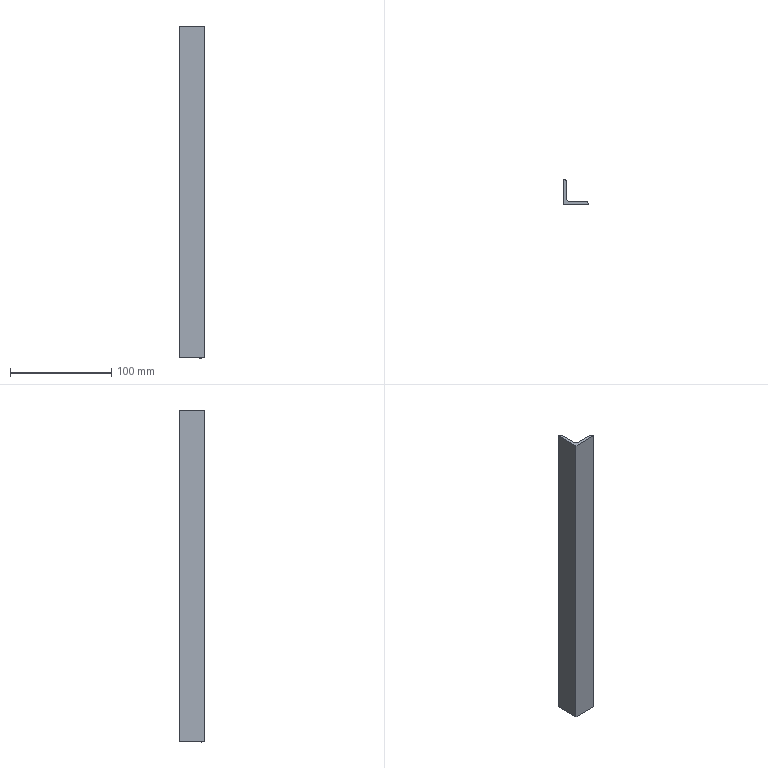Part | SolidWorks | features BaseBody 1 | 1 solid | 9 faces | box 25 x 25 x 328 mm | volume 45614 mm3 | plane 6 | cylinder 3 | commonest cylinder face diameters 6 x3
STEP:
#1=CARTESIAN_POINT('',(3.,22.,164.));
#2=VERTEX_POINT('',#1);
#3=CARTESIAN_POINT('',(0.,25.,164.));
#4=VERTEX_POINT('',#3);
#5=CARTESIAN_POINT('',(0.,22.,164.));
#6=DIRECTION('',(0.,0.,1.));
#7=DIRECTION('',(-1.,0.,0.));
#8=AXIS2_PLACEMENT_3D('',#5,#6,#7);
#9=CIRCLE('',#8,3.);
#10=EDGE_CURVE('',#2,#4,#9,.T.);
#11=ORIENTED_EDGE('',*,*,#10,.F.);
#12=CARTESIAN_POINT('',(3.,22.,-164.));
#13=VERTEX_POINT('',#12);
#14=CARTESIAN_POINT('',(3.,22.,164.));
#15=DIRECTION('',(0.,0.,1.));
#16=VECTOR('',#15,1000.);
#17=LINE('',#14,#16);
#18=EDGE_CURVE('',#13,#2,#17,.T.);
#19=ORIENTED_EDGE('',*,*,#18,.F.);
#20=CARTESIAN_POINT('',(0.,25.,-164.));
#21=VERTEX_POINT('',#20);
#22=CARTESIAN_POINT('',(0.,22.,-164.));
#23=DIRECTION('',(0.,0.,-1.));
#24=DIRECTION('',(-1.,0.,0.));
#25=AXIS2_PLACEMENT_3D('',#22,#23,#24);
#26=CIRCLE('',#25,3.);
#27=EDGE_CURVE('',#21,#13,#26,.T.);
#28=ORIENTED_EDGE('',*,*,#27,.F.);
#29=CARTESIAN_POINT('',(0.,25.,164.));
#30=DIRECTION('',(0.,0.,-1.));
#31=VECTOR('',#30,1000.);
#32=LINE('',#29,#31);
#33=EDGE_CURVE('',#4,#21,#32,.T.);
#34=ORIENTED_EDGE('',*,*,#33,.F.);
#35=EDGE_LOOP('',(#11,#19,#28,#34));
#36=FACE_OUTER_BOUND('',#35,.T.);
#37=CARTESIAN_POINT('',(0.,22.,164.));
#38=DIRECTION('',(0.,0.,-1.));
#39=DIRECTION('',(-1.,0.,0.));
#40=AXIS2_PLACEMENT_3D('',#37,#38,#39);
#41=CYLINDRICAL_SURFACE('',#40,3.);
#42=ADVANCED_FACE('',(#36),#41,.T.);
#43=CARTESIAN_POINT('',(25.,0.,164.));
#44=VERTEX_POINT('',#43);
#45=CARTESIAN_POINT('',(22.,3.,164.));
#46=VERTEX_POINT('',#45);
#47=CARTESIAN_POINT('',(22.,0.,164.));
#48=DIRECTION('',(0.,0.,1.));
#49=DIRECTION('',(-1.,0.,0.));
#50=AXIS2_PLACEMENT_3D('',#47,#48,#49);
#51=CIRCLE('',#50,3.);
#52=EDGE_CURVE('',#44,#46,#51,.T.);
#53=ORIENTED_EDGE('',*,*,#52,.F.);
#54=CARTESIAN_POINT('',(25.,0.,-164.));
#55=VERTEX_POINT('',#54);
#56=CARTESIAN_POINT('',(25.,0.,164.));
#57=DIRECTION('',(0.,0.,-1.));
#58=VECTOR('',#57,1000.);
#59=LINE('',#56,#58);
#60=EDGE_CURVE('',#44,#55,#59,.T.);
#61=ORIENTED_EDGE('',*,*,#60,.T.);
#62=CARTESIAN_POINT('',(22.,3.,-164.));
#63=VERTEX_POINT('',#62);
#64=CARTESIAN_POINT('',(22.,0.,-164.));
#65=DIRECTION('',(0.,0.,-1.));
#66=DIRECTION('',(-1.,0.,0.));
#67=AXIS2_PLACEMENT_3D('',#64,#65,#66);
#68=CIRCLE('',#67,3.);
#69=EDGE_CURVE('',#63,#55,#68,.T.);
#70=ORIENTED_EDGE('',*,*,#69,.F.);
#71=CARTESIAN_POINT('',(22.,3.,164.));
#72=DIRECTION('',(0.,0.,-1.));
#73=VECTOR('',#72,1000.);
#74=LINE('',#71,#73);
#75=EDGE_CURVE('',#46,#63,#74,.T.);
#76=ORIENTED_EDGE('',*,*,#75,.F.);
#77=EDGE_LOOP('',(#53,#61,#70,#76));
#78=FACE_OUTER_BOUND('',#77,.T.);
#79=CARTESIAN_POINT('',(22.,0.,164.));
#80=DIRECTION('',(0.,0.,-1.));
#81=DIRECTION('',(-1.,0.,0.));
#82=AXIS2_PLACEMENT_3D('',#79,#80,#81);
#83=CYLINDRICAL_SURFACE('',#82,3.);
#84=ADVANCED_FACE('',(#78),#83,.T.);
#85=CARTESIAN_POINT('',(6.,3.,164.));
#86=VERTEX_POINT('',#85);
#87=CARTESIAN_POINT('',(3.,6.,164.));
#88=VERTEX_POINT('',#87);
#89=CARTESIAN_POINT('',(6.,6.,164.));
#90=DIRECTION('',(0.,0.,-1.));
#91=DIRECTION('',(-1.,0.,0.));
#92=AXIS2_PLACEMENT_3D('',#89,#90,#91);
#93=CIRCLE('',#92,3.);
#94=EDGE_CURVE('',#86,#88,#93,.T.);
#95=ORIENTED_EDGE('',*,*,#94,.F.);
#96=CARTESIAN_POINT('',(6.,3.,-164.));
#97=VERTEX_POINT('',#96);
#98=CARTESIAN_POINT('',(6.,3.,164.));
#99=DIRECTION('',(0.,0.,1.));
#100=VECTOR('',#99,1000.);
#101=LINE('',#98,#100);
#102=EDGE_CURVE('',#97,#86,#101,.T.);
#103=ORIENTED_EDGE('',*,*,#102,.F.);
#104=CARTESIAN_POINT('',(3.,6.,-164.));
#105=VERTEX_POINT('',#104);
#106=CARTESIAN_POINT('',(6.,6.,-164.));
#107=DIRECTION('',(0.,0.,1.));
#108=DIRECTION('',(-1.,0.,0.));
#109=AXIS2_PLACEMENT_3D('',#106,#107,#108);
#110=CIRCLE('',#109,3.);
#111=EDGE_CURVE('',#105,#97,#110,.T.);
#112=ORIENTED_EDGE('',*,*,#111,.F.);
#113=CARTESIAN_POINT('',(3.,6.,-164.));
#114=DIRECTION('',(0.,0.,-1.));
#115=VECTOR('',#114,1000.);
#116=LINE('',#113,#115);
#117=EDGE_CURVE('',#88,#105,#116,.T.);
#118=ORIENTED_EDGE('',*,*,#117,.F.);
#119=EDGE_LOOP('',(#95,#103,#112,#118));
#120=FACE_OUTER_BOUND('',#119,.T.);
#121=CARTESIAN_POINT('',(6.,6.,164.));
#122=DIRECTION('',(0.,0.,1.));
#123=DIRECTION('',(1.,0.,0.));
#124=AXIS2_PLACEMENT_3D('',#121,#122,#123);
#125=CYLINDRICAL_SURFACE('',#124,3.);
#126=ADVANCED_FACE('',(#120),#125,.F.);
#127=CARTESIAN_POINT('',(3.,3.,-164.));
#128=DIRECTION('',(-1.,0.,0.));
#129=VECTOR('',#128,1000.);
#130=LINE('',#127,#129);
#131=EDGE_CURVE('',#63,#97,#130,.T.);
#132=ORIENTED_EDGE('',*,*,#131,.F.);
#133=ORIENTED_EDGE('',*,*,#69,.T.);
#134=CARTESIAN_POINT('',(0.,0.,-164.));
#135=VERTEX_POINT('',#134);
#136=CARTESIAN_POINT('',(0.,0.,-164.));
#137=DIRECTION('',(1.,0.,0.));
#138=VECTOR('',#137,1000.);
#139=LINE('',#136,#138);
#140=EDGE_CURVE('',#135,#55,#139,.T.);
#141=ORIENTED_EDGE('',*,*,#140,.F.);
#142=CARTESIAN_POINT('',(0.,0.,-164.));
#143=DIRECTION('',(0.,-1.,0.));
#144=VECTOR('',#143,1000.);
#145=LINE('',#142,#144);
#146=EDGE_CURVE('',#21,#135,#145,.T.);
#147=ORIENTED_EDGE('',*,*,#146,.F.);
#148=ORIENTED_EDGE('',*,*,#27,.T.);
#149=CARTESIAN_POINT('',(3.,25.,-164.));
#150=DIRECTION('',(0.,1.,0.));
#151=VECTOR('',#150,1000.);
#152=LINE('',#149,#151);
#153=EDGE_CURVE('',#105,#13,#152,.T.);
#154=ORIENTED_EDGE('',*,*,#153,.F.);
#155=ORIENTED_EDGE('',*,*,#111,.T.);
#156=EDGE_LOOP('',(#132,#133,#141,#147,#148,#154,#155));
#157=FACE_OUTER_BOUND('',#156,.T.);
#158=CARTESIAN_POINT('',(0.,0.,-164.));
#159=DIRECTION('',(0.,0.,-1.));
#160=DIRECTION('',(0.,-1.,0.));
#161=AXIS2_PLACEMENT_3D('',#158,#159,#160);
#162=PLANE('',#161);
#163=ADVANCED_FACE('',(#157),#162,.T.);
#164=CARTESIAN_POINT('',(0.,0.,164.));
#165=VERTEX_POINT('',#164);
#166=CARTESIAN_POINT('',(0.,0.,164.));
#167=DIRECTION('',(1.,0.,0.));
#168=VECTOR('',#167,1000.);
#169=LINE('',#166,#168);
#170=EDGE_CURVE('',#165,#44,#169,.T.);
#171=ORIENTED_EDGE('',*,*,#170,.T.);
#172=ORIENTED_EDGE('',*,*,#52,.T.);
#173=CARTESIAN_POINT('',(3.,3.,164.));
#174=DIRECTION('',(-1.,0.,0.));
#175=VECTOR('',#174,1000.);
#176=LINE('',#173,#175);
#177=EDGE_CURVE('',#46,#86,#176,.T.);
#178=ORIENTED_EDGE('',*,*,#177,.T.);
#179=ORIENTED_EDGE('',*,*,#94,.T.);
#180=CARTESIAN_POINT('',(3.,25.,164.));
#181=DIRECTION('',(0.,1.,0.));
#182=VECTOR('',#181,1000.);
#183=LINE('',#180,#182);
#184=EDGE_CURVE('',#88,#2,#183,.T.);
#185=ORIENTED_EDGE('',*,*,#184,.T.);
#186=ORIENTED_EDGE('',*,*,#10,.T.);
#187=CARTESIAN_POINT('',(0.,0.,164.));
#188=DIRECTION('',(0.,-1.,0.));
#189=VECTOR('',#188,1000.);
#190=LINE('',#187,#189);
#191=EDGE_CURVE('',#4,#165,#190,.T.);
#192=ORIENTED_EDGE('',*,*,#191,.T.);
#193=EDGE_LOOP('',(#171,#172,#178,#179,#185,#186,#192));
#194=FACE_OUTER_BOUND('',#193,.T.);
#195=CARTESIAN_POINT('',(0.,0.,164.));
#196=DIRECTION('',(0.,0.,-1.));
#197=DIRECTION('',(0.,-1.,0.));
#198=AXIS2_PLACEMENT_3D('',#195,#196,#197);
#199=PLANE('',#198);
#200=ADVANCED_FACE('',(#194),#199,.F.);
#201=ORIENTED_EDGE('',*,*,#153,.T.);
#202=ORIENTED_EDGE('',*,*,#18,.T.);
#203=ORIENTED_EDGE('',*,*,#184,.F.);
#204=ORIENTED_EDGE('',*,*,#117,.T.);
#205=EDGE_LOOP('',(#201,#202,#203,#204));
#206=FACE_OUTER_BOUND('',#205,.T.);
#207=CARTESIAN_POINT('',(3.,25.,164.));
#208=DIRECTION('',(-1.,0.,0.));
#209=DIRECTION('',(0.,1.,0.));
#210=AXIS2_PLACEMENT_3D('',#207,#208,#209);
#211=PLANE('',#210);
#212=ADVANCED_FACE('',(#206),#211,.F.);
#213=ORIENTED_EDGE('',*,*,#177,.F.);
#214=ORIENTED_EDGE('',*,*,#75,.T.);
#215=ORIENTED_EDGE('',*,*,#131,.T.);
#216=ORIENTED_EDGE('',*,*,#102,.T.);
#217=EDGE_LOOP('',(#213,#214,#215,#216));
#218=FACE_OUTER_BOUND('',#217,.T.);
#219=CARTESIAN_POINT('',(3.,3.,164.));
#220=DIRECTION('',(0.,-1.,0.));
#221=DIRECTION('',(0.,0.,-1.));
#222=AXIS2_PLACEMENT_3D('',#219,#220,#221);
#223=PLANE('',#222);
#224=ADVANCED_FACE('',(#218),#223,.F.);
#225=ORIENTED_EDGE('',*,*,#140,.T.);
#226=ORIENTED_EDGE('',*,*,#60,.F.);
#227=ORIENTED_EDGE('',*,*,#170,.F.);
#228=CARTESIAN_POINT('',(0.,0.,164.));
#229=DIRECTION('',(0.,0.,-1.));
#230=VECTOR('',#229,1000.);
#231=LINE('',#228,#230);
#232=EDGE_CURVE('',#165,#135,#231,.T.);
#233=ORIENTED_EDGE('',*,*,#232,.T.);
#234=EDGE_LOOP('',(#225,#226,#227,#233));
#235=FACE_OUTER_BOUND('',#234,.T.);
#236=CARTESIAN_POINT('',(0.,0.,164.));
#237=DIRECTION('',(0.,1.,0.));
#238=DIRECTION('',(1.,0.,0.));
#239=AXIS2_PLACEMENT_3D('',#236,#237,#238);
#240=PLANE('',#239);
#241=ADVANCED_FACE('',(#235),#240,.F.);
#242=ORIENTED_EDGE('',*,*,#146,.T.);
#243=ORIENTED_EDGE('',*,*,#232,.F.);
#244=ORIENTED_EDGE('',*,*,#191,.F.);
#245=ORIENTED_EDGE('',*,*,#33,.T.);
#246=EDGE_LOOP('',(#242,#243,#244,#245));
#247=FACE_OUTER_BOUND('',#246,.T.);
#248=CARTESIAN_POINT('',(0.,0.,164.));
#249=DIRECTION('',(1.,0.,0.));
#250=DIRECTION('',(0.,1.,0.));
#251=AXIS2_PLACEMENT_3D('',#248,#249,#250);
#252=PLANE('',#251);
#253=ADVANCED_FACE('',(#247),#252,.F.);
#254=CLOSED_SHELL('',(#42,#84,#126,#163,#200,#212,#224,#241,#253));
#255=MANIFOLD_SOLID_BREP('',#254);
#256=CARTESIAN_POINT('',(0.,0.,0.));
#257=DIRECTION('',(0.,0.,1.));
#258=DIRECTION('',(1.,0.,0.));
#259=AXIS2_PLACEMENT_3D('',#256,#257,#258);
#260=(LENGTH_UNIT()NAMED_UNIT(*)SI_UNIT(.MILLI.,.METRE.));
#261=UNCERTAINTY_MEASURE_WITH_UNIT(LENGTH_MEASURE(0.00001),#260,'','');
#262=(NAMED_UNIT(*)PLANE_ANGLE_UNIT()SI_UNIT($,.RADIAN.));
#263=(NAMED_UNIT(*)SI_UNIT($,.STERADIAN.)SOLID_ANGLE_UNIT());
#264=(GEOMETRIC_REPRESENTATION_CONTEXT(3)GLOBAL_UNCERTAINTY_ASSIGNED_CONTEXT((#261))GLOBAL_UNIT_ASSIGNED_CONTEXT((#260,#262,#263))REPRESENTATION_CONTEXT('',''));
#265=ADVANCED_BREP_SHAPE_REPRESENTATION('',(#255,#259),#264);